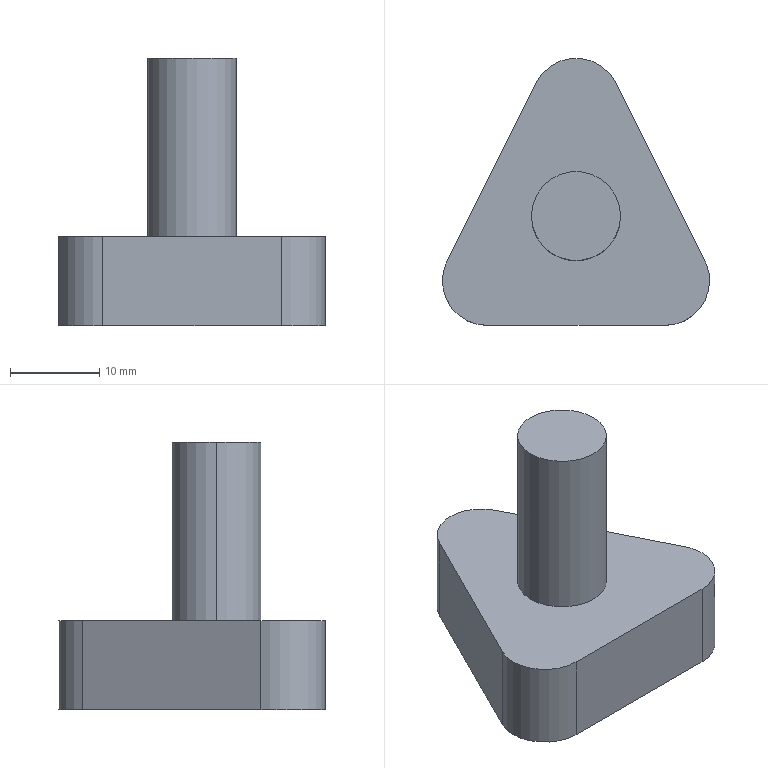Part | STEP file | 1 solid | 12 faces | box 30 x 30 x 30 mm | volume 7592 mm3 | cylinder 6 | plane 6 | commonest cylinder face diameters 10 x6
STEP:
#1=CARTESIAN_POINT('',(0.,0.,0.));
#2=DIRECTION('',(0.,0.,1.));
#3=DIRECTION('',(1.,0.,0.));
#4=AXIS2_PLACEMENT_3D('',#1,#2,#3);
#5=CARTESIAN_POINT('',(5.,-27.762,10.));
#6=VERTEX_POINT('',#5);
#7=CARTESIAN_POINT('',(-5.,-27.762,10.));
#8=VERTEX_POINT('',#7);
#9=CARTESIAN_POINT('',(0.,-27.762,10.));
#10=DIRECTION('',(0.,0.,1.));
#11=DIRECTION('',(1.,0.,0.));
#12=AXIS2_PLACEMENT_3D('',#9,#10,#11);
#13=CIRCLE('',#12,5.);
#14=CARTESIAN_POINT('',(0.,-27.762,10.));
#15=DIRECTION('',(0.,0.,1.));
#16=DIRECTION('',(1.,0.,0.));
#17=AXIS2_PLACEMENT_3D('',#14,#15,#16);
#18=CYLINDRICAL_SURFACE('',#17,5.);
#19=CARTESIAN_POINT('',(0.,0.));
#20=DIRECTION('',(1.,0.));
#21=VECTOR('',#20,1.);
#22=LINE('',#19,#21);
#23=(GEOMETRIC_REPRESENTATION_CONTEXT(2)PARAMETRIC_REPRESENTATION_CONTEXT()REPRESENTATION_CONTEXT('',''));
#24=DEFINITIONAL_REPRESENTATION('',(#22),#23);
#25=PCURVE('',#18,#24);
#26=CARTESIAN_POINT('',(0.,-28.053,10.));
#27=DIRECTION('',(0.,0.,1.));
#28=DIRECTION('',(1.,0.,0.));
#29=AXIS2_PLACEMENT_3D('',#26,#27,#28);
#30=PLANE('',#29);
#31=CARTESIAN_POINT('',(0.,0.2914));
#32=DIRECTION('',(1.,0.));
#33=AXIS2_PLACEMENT_2D('',#31,#32);
#34=CIRCLE('',#33,5.);
#35=(GEOMETRIC_REPRESENTATION_CONTEXT(2)PARAMETRIC_REPRESENTATION_CONTEXT()REPRESENTATION_CONTEXT('',''));
#36=DEFINITIONAL_REPRESENTATION('',(#34),#35);
#37=PCURVE('',#30,#36);
#38=SURFACE_CURVE('',#13,(#25,#37),.PCURVE_S1.);
#39=EDGE_CURVE('',#6,#8,#38,.T.);
#40=ORIENTED_EDGE('',*,*,#39,.T.);
#41=CARTESIAN_POINT('',(-5.,-27.762,30.));
#42=VERTEX_POINT('',#41);
#43=CARTESIAN_POINT('',(-5.,-27.762,10.));
#44=DIRECTION('',(0.,0.,1.));
#45=VECTOR('',#44,1.);
#46=LINE('',#43,#45);
#47=CARTESIAN_POINT('',(3.142,0.));
#48=DIRECTION('',(0.,1.));
#49=VECTOR('',#48,1.);
#50=LINE('',#47,#49);
#51=(GEOMETRIC_REPRESENTATION_CONTEXT(2)PARAMETRIC_REPRESENTATION_CONTEXT()REPRESENTATION_CONTEXT('',''));
#52=DEFINITIONAL_REPRESENTATION('',(#50),#51);
#53=PCURVE('',#18,#52);
#54=CARTESIAN_POINT('',(0.,-27.762,10.));
#55=DIRECTION('',(0.,0.,1.));
#56=DIRECTION('',(1.,0.,0.));
#57=AXIS2_PLACEMENT_3D('',#54,#55,#56);
#58=CYLINDRICAL_SURFACE('',#57,5.);
#59=CARTESIAN_POINT('',(3.142,0.));
#60=DIRECTION('',(0.,1.));
#61=VECTOR('',#60,1.);
#62=LINE('',#59,#61);
#63=(GEOMETRIC_REPRESENTATION_CONTEXT(2)PARAMETRIC_REPRESENTATION_CONTEXT()REPRESENTATION_CONTEXT('',''));
#64=DEFINITIONAL_REPRESENTATION('',(#62),#63);
#65=PCURVE('',#58,#64);
#66=SURFACE_CURVE('',#46,(#53,#65),.PCURVE_S1.);
#67=EDGE_CURVE('',#8,#42,#66,.T.);
#68=ORIENTED_EDGE('',*,*,#67,.T.);
#69=CARTESIAN_POINT('',(5.,-27.762,30.));
#70=VERTEX_POINT('',#69);
#71=CARTESIAN_POINT('',(0.,-27.762,30.));
#72=DIRECTION('',(0.,0.,-1.));
#73=DIRECTION('',(1.,0.,0.));
#74=AXIS2_PLACEMENT_3D('',#71,#72,#73);
#75=CIRCLE('',#74,5.);
#76=CARTESIAN_POINT('',(6.283,20.));
#77=DIRECTION('',(-1.,0.));
#78=VECTOR('',#77,1.);
#79=LINE('',#76,#78);
#80=(GEOMETRIC_REPRESENTATION_CONTEXT(2)PARAMETRIC_REPRESENTATION_CONTEXT()REPRESENTATION_CONTEXT('',''));
#81=DEFINITIONAL_REPRESENTATION('',(#79),#80);
#82=PCURVE('',#18,#81);
#83=CARTESIAN_POINT('',(0.,-27.762,30.));
#84=DIRECTION('',(0.,0.,1.));
#85=DIRECTION('',(1.,0.,0.));
#86=AXIS2_PLACEMENT_3D('',#83,#84,#85);
#87=PLANE('',#86);
#88=CARTESIAN_POINT('',(5.,0.));
#89=CARTESIAN_POINT('',(5.,-8.66));
#90=CARTESIAN_POINT('',(-2.5,-4.33));
#91=CARTESIAN_POINT('',(-10.,0.));
#92=CARTESIAN_POINT('',(-2.5,4.33));
#93=CARTESIAN_POINT('',(5.,8.66));
#94=CARTESIAN_POINT('',(5.,0.));
#95=(BOUNDED_CURVE()B_SPLINE_CURVE(2,(#88,#89,#90,#91,#92,#93,#94),.UNSPECIFIED.,.T.,.F.)B_SPLINE_CURVE_WITH_KNOTS((1,2,2,2,2,1),(-2.094,0.,2.094,4.189,6.283,8.378),.UNSPECIFIED.)CURVE()GEOMETRIC_REPRESENTATION_ITEM()RATIONAL_B_SPLINE_CURVE((1.,0.5,1.,0.5,1.,0.5,1.))REPRESENTATION_ITEM(''));
#96=(GEOMETRIC_REPRESENTATION_CONTEXT(2)PARAMETRIC_REPRESENTATION_CONTEXT()REPRESENTATION_CONTEXT('',''));
#97=DEFINITIONAL_REPRESENTATION('',(#95),#96);
#98=PCURVE('',#87,#97);
#99=SURFACE_CURVE('',#75,(#82,#98),.PCURVE_S1.);
#100=EDGE_CURVE('',#42,#70,#99,.T.);
#101=ORIENTED_EDGE('',*,*,#100,.T.);
#102=CARTESIAN_POINT('',(5.,-27.762,10.));
#103=DIRECTION('',(0.,0.,1.));
#104=VECTOR('',#103,1.);
#105=LINE('',#102,#104);
#106=CARTESIAN_POINT('',(0.,0.));
#107=DIRECTION('',(0.,1.));
#108=VECTOR('',#107,1.);
#109=LINE('',#106,#108);
#110=(GEOMETRIC_REPRESENTATION_CONTEXT(2)PARAMETRIC_REPRESENTATION_CONTEXT()REPRESENTATION_CONTEXT('',''));
#111=DEFINITIONAL_REPRESENTATION('',(#109),#110);
#112=PCURVE('',#18,#111);
#113=CARTESIAN_POINT('',(6.283,0.));
#114=DIRECTION('',(0.,1.));
#115=VECTOR('',#114,1.);
#116=LINE('',#113,#115);
#117=(GEOMETRIC_REPRESENTATION_CONTEXT(2)PARAMETRIC_REPRESENTATION_CONTEXT()REPRESENTATION_CONTEXT('',''));
#118=DEFINITIONAL_REPRESENTATION('',(#116),#117);
#119=PCURVE('',#58,#118);
#120=SURFACE_CURVE('',#105,(#112,#119),.PCURVE_S1.);
#121=EDGE_CURVE('',#6,#70,#120,.T.);
#122=ORIENTED_EDGE('',*,*,#121,.F.);
#123=EDGE_LOOP('',(#40,#68,#101,#122));
#124=FACE_BOUND('',#123,.T.);
#125=ADVANCED_FACE('',(#124),#18,.T.);
#126=CARTESIAN_POINT('',(10.,-40.,0.));
#127=VERTEX_POINT('',#126);
#128=CARTESIAN_POINT('',(15.,-35.,0.));
#129=VERTEX_POINT('',#128);
#130=CARTESIAN_POINT('',(10.,-35.,0.));
#131=DIRECTION('',(0.,0.,1.));
#132=DIRECTION('',(1.,0.,0.));
#133=AXIS2_PLACEMENT_3D('',#130,#131,#132);
#134=CIRCLE('',#133,5.);
#135=CARTESIAN_POINT('',(10.,-35.,0.));
#136=DIRECTION('',(0.,0.,1.));
#137=DIRECTION('',(1.,0.,0.));
#138=AXIS2_PLACEMENT_3D('',#135,#136,#137);
#139=CYLINDRICAL_SURFACE('',#138,5.);
#140=CARTESIAN_POINT('',(0.,0.));
#141=DIRECTION('',(1.,0.));
#142=VECTOR('',#141,1.);
#143=LINE('',#140,#142);
#144=(GEOMETRIC_REPRESENTATION_CONTEXT(2)PARAMETRIC_REPRESENTATION_CONTEXT()REPRESENTATION_CONTEXT('',''));
#145=DEFINITIONAL_REPRESENTATION('',(#143),#144);
#146=PCURVE('',#139,#145);
#147=CARTESIAN_POINT('',(0.,-28.053,0.));
#148=DIRECTION('',(0.,0.,1.));
#149=DIRECTION('',(1.,0.,0.));
#150=AXIS2_PLACEMENT_3D('',#147,#148,#149);
#151=PLANE('',#150);
#152=CARTESIAN_POINT('',(10.,-6.947));
#153=DIRECTION('',(1.,0.));
#154=AXIS2_PLACEMENT_2D('',#152,#153);
#155=CIRCLE('',#154,5.);
#156=(GEOMETRIC_REPRESENTATION_CONTEXT(2)PARAMETRIC_REPRESENTATION_CONTEXT()REPRESENTATION_CONTEXT('',''));
#157=DEFINITIONAL_REPRESENTATION('',(#155),#156);
#158=PCURVE('',#151,#157);
#159=SURFACE_CURVE('',#134,(#146,#158),.PCURVE_S1.);
#160=EDGE_CURVE('',#127,#129,#159,.T.);
#161=ORIENTED_EDGE('',*,*,#160,.T.);
#162=CARTESIAN_POINT('',(15.,-35.,10.));
#163=VERTEX_POINT('',#162);
#164=CARTESIAN_POINT('',(15.,-35.,0.));
#165=DIRECTION('',(0.,0.,1.));
#166=VECTOR('',#165,1.);
#167=LINE('',#164,#166);
#168=CARTESIAN_POINT('',(6.283,0.));
#169=DIRECTION('',(0.,1.));
#170=VECTOR('',#169,1.);
#171=LINE('',#168,#170);
#172=(GEOMETRIC_REPRESENTATION_CONTEXT(2)PARAMETRIC_REPRESENTATION_CONTEXT()REPRESENTATION_CONTEXT('',''));
#173=DEFINITIONAL_REPRESENTATION('',(#171),#172);
#174=PCURVE('',#139,#173);
#175=CARTESIAN_POINT('',(10.,-35.,0.));
#176=DIRECTION('',(0.,0.,1.));
#177=DIRECTION('',(1.,0.,0.));
#178=AXIS2_PLACEMENT_3D('',#175,#176,#177);
#179=CYLINDRICAL_SURFACE('',#178,5.);
#180=CARTESIAN_POINT('',(0.,0.));
#181=DIRECTION('',(0.,1.));
#182=VECTOR('',#181,1.);
#183=LINE('',#180,#182);
#184=(GEOMETRIC_REPRESENTATION_CONTEXT(2)PARAMETRIC_REPRESENTATION_CONTEXT()REPRESENTATION_CONTEXT('',''));
#185=DEFINITIONAL_REPRESENTATION('',(#183),#184);
#186=PCURVE('',#179,#185);
#187=SURFACE_CURVE('',#167,(#174,#186),.PCURVE_S1.);
#188=EDGE_CURVE('',#129,#163,#187,.T.);
#189=ORIENTED_EDGE('',*,*,#188,.T.);
#190=CARTESIAN_POINT('',(10.,-40.,10.));
#191=VERTEX_POINT('',#190);
#192=CARTESIAN_POINT('',(10.,-35.,10.));
#193=DIRECTION('',(0.,0.,1.));
#194=DIRECTION('',(1.,0.,0.));
#195=AXIS2_PLACEMENT_3D('',#192,#193,#194);
#196=CIRCLE('',#195,5.);
#197=CARTESIAN_POINT('',(0.,10.));
#198=DIRECTION('',(1.,0.));
#199=VECTOR('',#198,1.);
#200=LINE('',#197,#199);
#201=(GEOMETRIC_REPRESENTATION_CONTEXT(2)PARAMETRIC_REPRESENTATION_CONTEXT()REPRESENTATION_CONTEXT('',''));
#202=DEFINITIONAL_REPRESENTATION('',(#200),#201);
#203=PCURVE('',#139,#202);
#204=CARTESIAN_POINT('',(10.,-6.947));
#205=DIRECTION('',(1.,0.));
#206=AXIS2_PLACEMENT_2D('',#204,#205);
#207=CIRCLE('',#206,5.);
#208=(GEOMETRIC_REPRESENTATION_CONTEXT(2)PARAMETRIC_REPRESENTATION_CONTEXT()REPRESENTATION_CONTEXT('',''));
#209=DEFINITIONAL_REPRESENTATION('',(#207),#208);
#210=PCURVE('',#30,#209);
#211=SURFACE_CURVE('',#196,(#203,#210),.PCURVE_S1.);
#212=EDGE_CURVE('',#191,#163,#211,.T.);
#213=ORIENTED_EDGE('',*,*,#212,.F.);
#214=CARTESIAN_POINT('',(10.,-40.,0.));
#215=DIRECTION('',(0.,0.,-1.));
#216=VECTOR('',#215,1.);
#217=LINE('',#214,#216);
#218=CARTESIAN_POINT('',(4.712,0.));
#219=DIRECTION('',(0.,-1.));
#220=VECTOR('',#219,1.);
#221=LINE('',#218,#220);
#222=(GEOMETRIC_REPRESENTATION_CONTEXT(2)PARAMETRIC_REPRESENTATION_CONTEXT()REPRESENTATION_CONTEXT('',''));
#223=DEFINITIONAL_REPRESENTATION('',(#221),#222);
#224=PCURVE('',#139,#223);
#225=CARTESIAN_POINT('',(-10.,-40.,0.));
#226=DIRECTION('',(0.,-1.,0.));
#227=DIRECTION('',(0.,0.,-1.));
#228=AXIS2_PLACEMENT_3D('',#225,#226,#227);
#229=PLANE('',#228);
#230=CARTESIAN_POINT('',(0.,20.));
#231=DIRECTION('',(1.,0.));
#232=VECTOR('',#231,1.);
#233=LINE('',#230,#232);
#234=(GEOMETRIC_REPRESENTATION_CONTEXT(2)PARAMETRIC_REPRESENTATION_CONTEXT()REPRESENTATION_CONTEXT('',''));
#235=DEFINITIONAL_REPRESENTATION('',(#233),#234);
#236=PCURVE('',#229,#235);
#237=SURFACE_CURVE('',#217,(#224,#236),.PCURVE_S1.);
#238=EDGE_CURVE('',#191,#127,#237,.T.);
#239=ORIENTED_EDGE('',*,*,#238,.T.);
#240=EDGE_LOOP('',(#161,#189,#213,#239));
#241=FACE_BOUND('',#240,.T.);
#242=ADVANCED_FACE('',(#241),#139,.T.);
#243=ORIENTED_EDGE('',*,*,#67,.F.);
#244=CARTESIAN_POINT('',(0.,-27.762,10.));
#245=DIRECTION('',(0.,0.,1.));
#246=DIRECTION('',(1.,0.,0.));
#247=AXIS2_PLACEMENT_3D('',#244,#245,#246);
#248=CIRCLE('',#247,5.);
#249=CARTESIAN_POINT('',(0.,0.));
#250=DIRECTION('',(1.,0.));
#251=VECTOR('',#250,1.);
#252=LINE('',#249,#251);
#253=(GEOMETRIC_REPRESENTATION_CONTEXT(2)PARAMETRIC_REPRESENTATION_CONTEXT()REPRESENTATION_CONTEXT('',''));
#254=DEFINITIONAL_REPRESENTATION('',(#252),#253);
#255=PCURVE('',#58,#254);
#256=CARTESIAN_POINT('',(0.,0.2914));
#257=DIRECTION('',(1.,0.));
#258=AXIS2_PLACEMENT_2D('',#256,#257);
#259=CIRCLE('',#258,5.);
#260=(GEOMETRIC_REPRESENTATION_CONTEXT(2)PARAMETRIC_REPRESENTATION_CONTEXT()REPRESENTATION_CONTEXT('',''));
#261=DEFINITIONAL_REPRESENTATION('',(#259),#260);
#262=PCURVE('',#30,#261);
#263=SURFACE_CURVE('',#248,(#255,#262),.PCURVE_S1.);
#264=EDGE_CURVE('',#8,#6,#263,.T.);
#265=ORIENTED_EDGE('',*,*,#264,.T.);
#266=ORIENTED_EDGE('',*,*,#121,.T.);
#267=CARTESIAN_POINT('',(0.,-27.762,30.));
#268=DIRECTION('',(0.,0.,-1.));
#269=DIRECTION('',(1.,0.,0.));
#270=AXIS2_PLACEMENT_3D('',#267,#268,#269);
#271=CIRCLE('',#270,5.);
#272=CARTESIAN_POINT('',(6.283,20.));
#273=DIRECTION('',(-1.,0.));
#274=VECTOR('',#273,1.);
#275=LINE('',#272,#274);
#276=(GEOMETRIC_REPRESENTATION_CONTEXT(2)PARAMETRIC_REPRESENTATION_CONTEXT()REPRESENTATION_CONTEXT('',''));
#277=DEFINITIONAL_REPRESENTATION('',(#275),#276);
#278=PCURVE('',#58,#277);
#279=CARTESIAN_POINT('',(5.,0.));
#280=CARTESIAN_POINT('',(5.,-8.66));
#281=CARTESIAN_POINT('',(-2.5,-4.33));
#282=CARTESIAN_POINT('',(-10.,0.));
#283=CARTESIAN_POINT('',(-2.5,4.33));
#284=CARTESIAN_POINT('',(5.,8.66));
#285=CARTESIAN_POINT('',(5.,0.));
#286=(BOUNDED_CURVE()B_SPLINE_CURVE(2,(#279,#280,#281,#282,#283,#284,#285),.UNSPECIFIED.,.T.,.F.)B_SPLINE_CURVE_WITH_KNOTS((1,2,2,2,2,1),(-2.094,0.,2.094,4.189,6.283,8.378),.UNSPECIFIED.)CURVE()GEOMETRIC_REPRESENTATION_ITEM()RATIONAL_B_SPLINE_CURVE((1.,0.5,1.,0.5,1.,0.5,1.))REPRESENTATION_ITEM(''));
#287=(GEOMETRIC_REPRESENTATION_CONTEXT(2)PARAMETRIC_REPRESENTATION_CONTEXT()REPRESENTATION_CONTEXT('',''));
#288=DEFINITIONAL_REPRESENTATION('',(#286),#287);
#289=PCURVE('',#87,#288);
#290=SURFACE_CURVE('',#271,(#278,#289),.PCURVE_S1.);
#291=EDGE_CURVE('',#70,#42,#290,.T.);
#292=ORIENTED_EDGE('',*,*,#291,.T.);
#293=EDGE_LOOP('',(#243,#265,#266,#292));
#294=FACE_BOUND('',#293,.T.);
#295=ADVANCED_FACE('',(#294),#58,.T.);
#296=CARTESIAN_POINT('',(-10.,-40.,10.));
#297=VERTEX_POINT('',#296);
#298=CARTESIAN_POINT('',(0.,-40.,10.));
#299=DIRECTION('',(1.,0.,0.));
#300=VECTOR('',#299,1.);
#301=LINE('',#298,#300);
#302=CARTESIAN_POINT('',(0.,-11.947));
#303=DIRECTION('',(1.,0.));
#304=VECTOR('',#303,1.);
#305=LINE('',#302,#304);
#306=(GEOMETRIC_REPRESENTATION_CONTEXT(2)PARAMETRIC_REPRESENTATION_CONTEXT()REPRESENTATION_CONTEXT('',''));
#307=DEFINITIONAL_REPRESENTATION('',(#305),#306);
#308=PCURVE('',#30,#307);
#309=CARTESIAN_POINT('',(-10.,10.));
#310=DIRECTION('',(0.,1.));
#311=VECTOR('',#310,1.);
#312=LINE('',#309,#311);
#313=(GEOMETRIC_REPRESENTATION_CONTEXT(2)PARAMETRIC_REPRESENTATION_CONTEXT()REPRESENTATION_CONTEXT('',''));
#314=DEFINITIONAL_REPRESENTATION('',(#312),#313);
#315=PCURVE('',#229,#314);
#316=SURFACE_CURVE('',#301,(#308,#315),.PCURVE_S1.);
#317=EDGE_CURVE('',#297,#191,#316,.T.);
#318=ORIENTED_EDGE('',*,*,#317,.T.);
#319=ORIENTED_EDGE('',*,*,#212,.T.);
#320=CARTESIAN_POINT('',(14.472,-32.764,10.));
#321=VERTEX_POINT('',#320);
#322=CARTESIAN_POINT('',(10.,-35.,10.));
#323=DIRECTION('',(0.,0.,1.));
#324=DIRECTION('',(1.,0.,0.));
#325=AXIS2_PLACEMENT_3D('',#322,#323,#324);
#326=CIRCLE('',#325,5.);
#327=CARTESIAN_POINT('',(10.,-6.947));
#328=DIRECTION('',(1.,0.));
#329=AXIS2_PLACEMENT_2D('',#327,#328);
#330=CIRCLE('',#329,5.);
#331=(GEOMETRIC_REPRESENTATION_CONTEXT(2)PARAMETRIC_REPRESENTATION_CONTEXT()REPRESENTATION_CONTEXT('',''));
#332=DEFINITIONAL_REPRESENTATION('',(#330),#331);
#333=PCURVE('',#30,#332);
#334=CARTESIAN_POINT('',(0.,10.));
#335=DIRECTION('',(1.,0.));
#336=VECTOR('',#335,1.);
#337=LINE('',#334,#336);
#338=(GEOMETRIC_REPRESENTATION_CONTEXT(2)PARAMETRIC_REPRESENTATION_CONTEXT()REPRESENTATION_CONTEXT('',''));
#339=DEFINITIONAL_REPRESENTATION('',(#337),#338);
#340=PCURVE('',#179,#339);
#341=SURFACE_CURVE('',#326,(#333,#340),.PCURVE_S1.);
#342=EDGE_CURVE('',#163,#321,#341,.T.);
#343=ORIENTED_EDGE('',*,*,#342,.T.);
#344=CARTESIAN_POINT('',(4.472,-12.764,10.));
#345=VERTEX_POINT('',#344);
#346=CARTESIAN_POINT('',(14.472,-32.764,10.));
#347=DIRECTION('',(-0.4472,0.8944,0.));
#348=VECTOR('',#347,1.);
#349=LINE('',#346,#348);
#350=CARTESIAN_POINT('',(14.472,-4.711));
#351=DIRECTION('',(-0.4472,0.8944));
#352=VECTOR('',#351,1.);
#353=LINE('',#350,#352);
#354=(GEOMETRIC_REPRESENTATION_CONTEXT(2)PARAMETRIC_REPRESENTATION_CONTEXT()REPRESENTATION_CONTEXT('',''));
#355=DEFINITIONAL_REPRESENTATION('',(#353),#354);
#356=PCURVE('',#30,#355);
#357=CARTESIAN_POINT('',(14.472,-32.764,0.));
#358=DIRECTION('',(0.8944,0.4472,0.));
#359=DIRECTION('',(-0.4472,0.8944,0.));
#360=AXIS2_PLACEMENT_3D('',#357,#358,#359);
#361=PLANE('',#360);
#362=CARTESIAN_POINT('',(0.,10.));
#363=DIRECTION('',(1.,0.));
#364=VECTOR('',#363,1.);
#365=LINE('',#362,#364);
#366=(GEOMETRIC_REPRESENTATION_CONTEXT(2)PARAMETRIC_REPRESENTATION_CONTEXT()REPRESENTATION_CONTEXT('',''));
#367=DEFINITIONAL_REPRESENTATION('',(#365),#366);
#368=PCURVE('',#361,#367);
#369=SURFACE_CURVE('',#349,(#356,#368),.PCURVE_S1.);
#370=EDGE_CURVE('',#321,#345,#369,.T.);
#371=ORIENTED_EDGE('',*,*,#370,.T.);
#372=CARTESIAN_POINT('',(-4.472,-12.764,10.));
#373=VERTEX_POINT('',#372);
#374=CARTESIAN_POINT('',(0.,-15.,10.));
#375=DIRECTION('',(0.,0.,1.));
#376=DIRECTION('',(1.,0.,0.));
#377=AXIS2_PLACEMENT_3D('',#374,#375,#376);
#378=CIRCLE('',#377,5.);
#379=CARTESIAN_POINT('',(0.,13.053));
#380=DIRECTION('',(1.,0.));
#381=AXIS2_PLACEMENT_2D('',#379,#380);
#382=CIRCLE('',#381,5.);
#383=(GEOMETRIC_REPRESENTATION_CONTEXT(2)PARAMETRIC_REPRESENTATION_CONTEXT()REPRESENTATION_CONTEXT('',''));
#384=DEFINITIONAL_REPRESENTATION('',(#382),#383);
#385=PCURVE('',#30,#384);
#386=CARTESIAN_POINT('',(0.,-15.,0.));
#387=DIRECTION('',(0.,0.,1.));
#388=DIRECTION('',(1.,0.,0.));
#389=AXIS2_PLACEMENT_3D('',#386,#387,#388);
#390=CYLINDRICAL_SURFACE('',#389,5.);
#391=CARTESIAN_POINT('',(0.,10.));
#392=DIRECTION('',(1.,0.));
#393=VECTOR('',#392,1.);
#394=LINE('',#391,#393);
#395=(GEOMETRIC_REPRESENTATION_CONTEXT(2)PARAMETRIC_REPRESENTATION_CONTEXT()REPRESENTATION_CONTEXT('',''));
#396=DEFINITIONAL_REPRESENTATION('',(#394),#395);
#397=PCURVE('',#390,#396);
#398=SURFACE_CURVE('',#378,(#385,#397),.PCURVE_S1.);
#399=EDGE_CURVE('',#345,#373,#398,.T.);
#400=ORIENTED_EDGE('',*,*,#399,.T.);
#401=CARTESIAN_POINT('',(-14.472,-32.764,10.));
#402=VERTEX_POINT('',#401);
#403=CARTESIAN_POINT('',(-4.472,-12.764,10.));
#404=DIRECTION('',(-0.4472,-0.8944,0.));
#405=VECTOR('',#404,1.);
#406=LINE('',#403,#405);
#407=CARTESIAN_POINT('',(-4.472,15.289));
#408=DIRECTION('',(-0.4472,-0.8944));
#409=VECTOR('',#408,1.);
#410=LINE('',#407,#409);
#411=(GEOMETRIC_REPRESENTATION_CONTEXT(2)PARAMETRIC_REPRESENTATION_CONTEXT()REPRESENTATION_CONTEXT('',''));
#412=DEFINITIONAL_REPRESENTATION('',(#410),#411);
#413=PCURVE('',#30,#412);
#414=CARTESIAN_POINT('',(-4.472,-12.764,0.));
#415=DIRECTION('',(-0.8944,0.4472,0.));
#416=DIRECTION('',(-0.4472,-0.8944,0.));
#417=AXIS2_PLACEMENT_3D('',#414,#415,#416);
#418=PLANE('',#417);
#419=CARTESIAN_POINT('',(0.,10.));
#420=DIRECTION('',(1.,0.));
#421=VECTOR('',#420,1.);
#422=LINE('',#419,#421);
#423=(GEOMETRIC_REPRESENTATION_CONTEXT(2)PARAMETRIC_REPRESENTATION_CONTEXT()REPRESENTATION_CONTEXT('',''));
#424=DEFINITIONAL_REPRESENTATION('',(#422),#423);
#425=PCURVE('',#418,#424);
#426=SURFACE_CURVE('',#406,(#413,#425),.PCURVE_S1.);
#427=EDGE_CURVE('',#373,#402,#426,.T.);
#428=ORIENTED_EDGE('',*,*,#427,.T.);
#429=CARTESIAN_POINT('',(-10.,-35.,10.));
#430=DIRECTION('',(0.,0.,1.));
#431=DIRECTION('',(1.,0.,0.));
#432=AXIS2_PLACEMENT_3D('',#429,#430,#431);
#433=CIRCLE('',#432,5.);
#434=CARTESIAN_POINT('',(-10.,-6.947));
#435=DIRECTION('',(1.,0.));
#436=AXIS2_PLACEMENT_2D('',#434,#435);
#437=CIRCLE('',#436,5.);
#438=(GEOMETRIC_REPRESENTATION_CONTEXT(2)PARAMETRIC_REPRESENTATION_CONTEXT()REPRESENTATION_CONTEXT('',''));
#439=DEFINITIONAL_REPRESENTATION('',(#437),#438);
#440=PCURVE('',#30,#439);
#441=CARTESIAN_POINT('',(-10.,-35.,0.));
#442=DIRECTION('',(0.,0.,1.));
#443=DIRECTION('',(1.,0.,0.));
#444=AXIS2_PLACEMENT_3D('',#441,#442,#443);
#445=CYLINDRICAL_SURFACE('',#444,5.);
#446=CARTESIAN_POINT('',(0.,10.));
#447=DIRECTION('',(1.,0.));
#448=VECTOR('',#447,1.);
#449=LINE('',#446,#448);
#450=(GEOMETRIC_REPRESENTATION_CONTEXT(2)PARAMETRIC_REPRESENTATION_CONTEXT()REPRESENTATION_CONTEXT('',''));
#451=DEFINITIONAL_REPRESENTATION('',(#449),#450);
#452=PCURVE('',#445,#451);
#453=SURFACE_CURVE('',#433,(#440,#452),.PCURVE_S1.);
#454=EDGE_CURVE('',#402,#297,#453,.T.);
#455=ORIENTED_EDGE('',*,*,#454,.T.);
#456=EDGE_LOOP('',(#318,#319,#343,#371,#400,#428,#455));
#457=FACE_BOUND('',#456,.T.);
#458=ORIENTED_EDGE('',*,*,#39,.F.);
#459=ORIENTED_EDGE('',*,*,#264,.F.);
#460=EDGE_LOOP('',(#458,#459));
#461=FACE_BOUND('',#460,.T.);
#462=ADVANCED_FACE('',(#457,#461),#30,.T.);
#463=ORIENTED_EDGE('',*,*,#291,.F.);
#464=ORIENTED_EDGE('',*,*,#100,.F.);
#465=EDGE_LOOP('',(#463,#464));
#466=FACE_BOUND('',#465,.T.);
#467=ADVANCED_FACE('',(#466),#87,.T.);
#468=ORIENTED_EDGE('',*,*,#188,.F.);
#469=CARTESIAN_POINT('',(14.472,-32.764,0.));
#470=VERTEX_POINT('',#469);
#471=CARTESIAN_POINT('',(10.,-35.,0.));
#472=DIRECTION('',(0.,0.,1.));
#473=DIRECTION('',(1.,0.,0.));
#474=AXIS2_PLACEMENT_3D('',#471,#472,#473);
#475=CIRCLE('',#474,5.);
#476=CARTESIAN_POINT('',(0.,0.));
#477=DIRECTION('',(1.,0.));
#478=VECTOR('',#477,1.);
#479=LINE('',#476,#478);
#480=(GEOMETRIC_REPRESENTATION_CONTEXT(2)PARAMETRIC_REPRESENTATION_CONTEXT()REPRESENTATION_CONTEXT('',''));
#481=DEFINITIONAL_REPRESENTATION('',(#479),#480);
#482=PCURVE('',#179,#481);
#483=CARTESIAN_POINT('',(10.,-6.947));
#484=DIRECTION('',(1.,0.));
#485=AXIS2_PLACEMENT_2D('',#483,#484);
#486=CIRCLE('',#485,5.);
#487=(GEOMETRIC_REPRESENTATION_CONTEXT(2)PARAMETRIC_REPRESENTATION_CONTEXT()REPRESENTATION_CONTEXT('',''));
#488=DEFINITIONAL_REPRESENTATION('',(#486),#487);
#489=PCURVE('',#151,#488);
#490=SURFACE_CURVE('',#475,(#482,#489),.PCURVE_S1.);
#491=EDGE_CURVE('',#129,#470,#490,.T.);
#492=ORIENTED_EDGE('',*,*,#491,.T.);
#493=CARTESIAN_POINT('',(14.472,-32.764,0.));
#494=DIRECTION('',(0.,0.,1.));
#495=VECTOR('',#494,1.);
#496=LINE('',#493,#495);
#497=CARTESIAN_POINT('',(0.4636,0.));
#498=DIRECTION('',(0.,1.));
#499=VECTOR('',#498,1.);
#500=LINE('',#497,#499);
#501=(GEOMETRIC_REPRESENTATION_CONTEXT(2)PARAMETRIC_REPRESENTATION_CONTEXT()REPRESENTATION_CONTEXT('',''));
#502=DEFINITIONAL_REPRESENTATION('',(#500),#501);
#503=PCURVE('',#179,#502);
#504=CARTESIAN_POINT('',(0.,0.));
#505=DIRECTION('',(0.,1.));
#506=VECTOR('',#505,1.);
#507=LINE('',#504,#506);
#508=(GEOMETRIC_REPRESENTATION_CONTEXT(2)PARAMETRIC_REPRESENTATION_CONTEXT()REPRESENTATION_CONTEXT('',''));
#509=DEFINITIONAL_REPRESENTATION('',(#507),#508);
#510=PCURVE('',#361,#509);
#511=SURFACE_CURVE('',#496,(#503,#510),.PCURVE_S1.);
#512=EDGE_CURVE('',#470,#321,#511,.T.);
#513=ORIENTED_EDGE('',*,*,#512,.T.);
#514=ORIENTED_EDGE('',*,*,#342,.F.);
#515=EDGE_LOOP('',(#468,#492,#513,#514));
#516=FACE_BOUND('',#515,.T.);
#517=ADVANCED_FACE('',(#516),#179,.T.);
#518=ORIENTED_EDGE('',*,*,#317,.F.);
#519=CARTESIAN_POINT('',(-10.,-40.,0.));
#520=VERTEX_POINT('',#519);
#521=CARTESIAN_POINT('',(-10.,-40.,0.));
#522=DIRECTION('',(0.,0.,-1.));
#523=VECTOR('',#522,1.);
#524=LINE('',#521,#523);
#525=CARTESIAN_POINT('',(0.,0.));
#526=DIRECTION('',(1.,0.));
#527=VECTOR('',#526,1.);
#528=LINE('',#525,#527);
#529=(GEOMETRIC_REPRESENTATION_CONTEXT(2)PARAMETRIC_REPRESENTATION_CONTEXT()REPRESENTATION_CONTEXT('',''));
#530=DEFINITIONAL_REPRESENTATION('',(#528),#529);
#531=PCURVE('',#229,#530);
#532=CARTESIAN_POINT('',(4.712,0.));
#533=DIRECTION('',(0.,-1.));
#534=VECTOR('',#533,1.);
#535=LINE('',#532,#534);
#536=(GEOMETRIC_REPRESENTATION_CONTEXT(2)PARAMETRIC_REPRESENTATION_CONTEXT()REPRESENTATION_CONTEXT('',''));
#537=DEFINITIONAL_REPRESENTATION('',(#535),#536);
#538=PCURVE('',#445,#537);
#539=SURFACE_CURVE('',#524,(#531,#538),.PCURVE_S1.);
#540=EDGE_CURVE('',#297,#520,#539,.T.);
#541=ORIENTED_EDGE('',*,*,#540,.T.);
#542=CARTESIAN_POINT('',(-10.,-40.,0.));
#543=DIRECTION('',(1.,0.,0.));
#544=VECTOR('',#543,1.);
#545=LINE('',#542,#544);
#546=CARTESIAN_POINT('',(0.,0.));
#547=DIRECTION('',(0.,1.));
#548=VECTOR('',#547,1.);
#549=LINE('',#546,#548);
#550=(GEOMETRIC_REPRESENTATION_CONTEXT(2)PARAMETRIC_REPRESENTATION_CONTEXT()REPRESENTATION_CONTEXT('',''));
#551=DEFINITIONAL_REPRESENTATION('',(#549),#550);
#552=PCURVE('',#229,#551);
#553=CARTESIAN_POINT('',(-10.,-11.947));
#554=DIRECTION('',(1.,0.));
#555=VECTOR('',#554,1.);
#556=LINE('',#553,#555);
#557=(GEOMETRIC_REPRESENTATION_CONTEXT(2)PARAMETRIC_REPRESENTATION_CONTEXT()REPRESENTATION_CONTEXT('',''));
#558=DEFINITIONAL_REPRESENTATION('',(#556),#557);
#559=PCURVE('',#151,#558);
#560=SURFACE_CURVE('',#545,(#552,#559),.PCURVE_S1.);
#561=EDGE_CURVE('',#520,#127,#560,.T.);
#562=ORIENTED_EDGE('',*,*,#561,.T.);
#563=ORIENTED_EDGE('',*,*,#238,.F.);
#564=EDGE_LOOP('',(#518,#541,#562,#563));
#565=FACE_BOUND('',#564,.T.);
#566=ADVANCED_FACE('',(#565),#229,.T.);
#567=ORIENTED_EDGE('',*,*,#454,.F.);
#568=CARTESIAN_POINT('',(-14.472,-32.764,0.));
#569=VERTEX_POINT('',#568);
#570=CARTESIAN_POINT('',(-14.472,-32.764,0.));
#571=DIRECTION('',(0.,0.,-1.));
#572=VECTOR('',#571,1.);
#573=LINE('',#570,#572);
#574=CARTESIAN_POINT('',(2.678,0.));
#575=DIRECTION('',(0.,-1.));
#576=VECTOR('',#575,1.);
#577=LINE('',#574,#576);
#578=(GEOMETRIC_REPRESENTATION_CONTEXT(2)PARAMETRIC_REPRESENTATION_CONTEXT()REPRESENTATION_CONTEXT('',''));
#579=DEFINITIONAL_REPRESENTATION('',(#577),#578);
#580=PCURVE('',#445,#579);
#581=CARTESIAN_POINT('',(22.361,0.));
#582=DIRECTION('',(0.,-1.));
#583=VECTOR('',#582,1.);
#584=LINE('',#581,#583);
#585=(GEOMETRIC_REPRESENTATION_CONTEXT(2)PARAMETRIC_REPRESENTATION_CONTEXT()REPRESENTATION_CONTEXT('',''));
#586=DEFINITIONAL_REPRESENTATION('',(#584),#585);
#587=PCURVE('',#418,#586);
#588=SURFACE_CURVE('',#573,(#580,#587),.PCURVE_S1.);
#589=EDGE_CURVE('',#402,#569,#588,.T.);
#590=ORIENTED_EDGE('',*,*,#589,.T.);
#591=CARTESIAN_POINT('',(-10.,-35.,0.));
#592=DIRECTION('',(0.,0.,1.));
#593=DIRECTION('',(1.,0.,0.));
#594=AXIS2_PLACEMENT_3D('',#591,#592,#593);
#595=CIRCLE('',#594,5.);
#596=CARTESIAN_POINT('',(0.,0.));
#597=DIRECTION('',(1.,0.));
#598=VECTOR('',#597,1.);
#599=LINE('',#596,#598);
#600=(GEOMETRIC_REPRESENTATION_CONTEXT(2)PARAMETRIC_REPRESENTATION_CONTEXT()REPRESENTATION_CONTEXT('',''));
#601=DEFINITIONAL_REPRESENTATION('',(#599),#600);
#602=PCURVE('',#445,#601);
#603=CARTESIAN_POINT('',(-10.,-6.947));
#604=DIRECTION('',(1.,0.));
#605=AXIS2_PLACEMENT_2D('',#603,#604);
#606=CIRCLE('',#605,5.);
#607=(GEOMETRIC_REPRESENTATION_CONTEXT(2)PARAMETRIC_REPRESENTATION_CONTEXT()REPRESENTATION_CONTEXT('',''));
#608=DEFINITIONAL_REPRESENTATION('',(#606),#607);
#609=PCURVE('',#151,#608);
#610=SURFACE_CURVE('',#595,(#602,#609),.PCURVE_S1.);
#611=EDGE_CURVE('',#569,#520,#610,.T.);
#612=ORIENTED_EDGE('',*,*,#611,.T.);
#613=ORIENTED_EDGE('',*,*,#540,.F.);
#614=EDGE_LOOP('',(#567,#590,#612,#613));
#615=FACE_BOUND('',#614,.T.);
#616=ADVANCED_FACE('',(#615),#445,.T.);
#617=ORIENTED_EDGE('',*,*,#427,.F.);
#618=CARTESIAN_POINT('',(-4.472,-12.764,0.));
#619=VERTEX_POINT('',#618);
#620=CARTESIAN_POINT('',(-4.472,-12.764,0.));
#621=DIRECTION('',(0.,0.,-1.));
#622=VECTOR('',#621,1.);
#623=LINE('',#620,#622);
#624=CARTESIAN_POINT('',(0.,0.));
#625=DIRECTION('',(0.,-1.));
#626=VECTOR('',#625,1.);
#627=LINE('',#624,#626);
#628=(GEOMETRIC_REPRESENTATION_CONTEXT(2)PARAMETRIC_REPRESENTATION_CONTEXT()REPRESENTATION_CONTEXT('',''));
#629=DEFINITIONAL_REPRESENTATION('',(#627),#628);
#630=PCURVE('',#418,#629);
#631=CARTESIAN_POINT('',(2.678,0.));
#632=DIRECTION('',(0.,-1.));
#633=VECTOR('',#632,1.);
#634=LINE('',#631,#633);
#635=(GEOMETRIC_REPRESENTATION_CONTEXT(2)PARAMETRIC_REPRESENTATION_CONTEXT()REPRESENTATION_CONTEXT('',''));
#636=DEFINITIONAL_REPRESENTATION('',(#634),#635);
#637=PCURVE('',#390,#636);
#638=SURFACE_CURVE('',#623,(#630,#637),.PCURVE_S1.);
#639=EDGE_CURVE('',#373,#619,#638,.T.);
#640=ORIENTED_EDGE('',*,*,#639,.T.);
#641=CARTESIAN_POINT('',(-4.472,-12.764,0.));
#642=DIRECTION('',(-0.4472,-0.8944,0.));
#643=VECTOR('',#642,1.);
#644=LINE('',#641,#643);
#645=CARTESIAN_POINT('',(0.,0.));
#646=DIRECTION('',(1.,0.));
#647=VECTOR('',#646,1.);
#648=LINE('',#645,#647);
#649=(GEOMETRIC_REPRESENTATION_CONTEXT(2)PARAMETRIC_REPRESENTATION_CONTEXT()REPRESENTATION_CONTEXT('',''));
#650=DEFINITIONAL_REPRESENTATION('',(#648),#649);
#651=PCURVE('',#418,#650);
#652=CARTESIAN_POINT('',(-4.472,15.289));
#653=DIRECTION('',(-0.4472,-0.8944));
#654=VECTOR('',#653,1.);
#655=LINE('',#652,#654);
#656=(GEOMETRIC_REPRESENTATION_CONTEXT(2)PARAMETRIC_REPRESENTATION_CONTEXT()REPRESENTATION_CONTEXT('',''));
#657=DEFINITIONAL_REPRESENTATION('',(#655),#656);
#658=PCURVE('',#151,#657);
#659=SURFACE_CURVE('',#644,(#651,#658),.PCURVE_S1.);
#660=EDGE_CURVE('',#619,#569,#659,.T.);
#661=ORIENTED_EDGE('',*,*,#660,.T.);
#662=ORIENTED_EDGE('',*,*,#589,.F.);
#663=EDGE_LOOP('',(#617,#640,#661,#662));
#664=FACE_BOUND('',#663,.T.);
#665=ADVANCED_FACE('',(#664),#418,.T.);
#666=ORIENTED_EDGE('',*,*,#399,.F.);
#667=CARTESIAN_POINT('',(4.472,-12.764,0.));
#668=VERTEX_POINT('',#667);
#669=CARTESIAN_POINT('',(4.472,-12.764,0.));
#670=DIRECTION('',(0.,0.,-1.));
#671=VECTOR('',#670,1.);
#672=LINE('',#669,#671);
#673=CARTESIAN_POINT('',(0.4636,0.));
#674=DIRECTION('',(0.,-1.));
#675=VECTOR('',#674,1.);
#676=LINE('',#673,#675);
#677=(GEOMETRIC_REPRESENTATION_CONTEXT(2)PARAMETRIC_REPRESENTATION_CONTEXT()REPRESENTATION_CONTEXT('',''));
#678=DEFINITIONAL_REPRESENTATION('',(#676),#677);
#679=PCURVE('',#390,#678);
#680=CARTESIAN_POINT('',(22.361,0.));
#681=DIRECTION('',(0.,-1.));
#682=VECTOR('',#681,1.);
#683=LINE('',#680,#682);
#684=(GEOMETRIC_REPRESENTATION_CONTEXT(2)PARAMETRIC_REPRESENTATION_CONTEXT()REPRESENTATION_CONTEXT('',''));
#685=DEFINITIONAL_REPRESENTATION('',(#683),#684);
#686=PCURVE('',#361,#685);
#687=SURFACE_CURVE('',#672,(#679,#686),.PCURVE_S1.);
#688=EDGE_CURVE('',#345,#668,#687,.T.);
#689=ORIENTED_EDGE('',*,*,#688,.T.);
#690=CARTESIAN_POINT('',(0.,-15.,0.));
#691=DIRECTION('',(0.,0.,1.));
#692=DIRECTION('',(1.,0.,0.));
#693=AXIS2_PLACEMENT_3D('',#690,#691,#692);
#694=CIRCLE('',#693,5.);
#695=CARTESIAN_POINT('',(0.,0.));
#696=DIRECTION('',(1.,0.));
#697=VECTOR('',#696,1.);
#698=LINE('',#695,#697);
#699=(GEOMETRIC_REPRESENTATION_CONTEXT(2)PARAMETRIC_REPRESENTATION_CONTEXT()REPRESENTATION_CONTEXT('',''));
#700=DEFINITIONAL_REPRESENTATION('',(#698),#699);
#701=PCURVE('',#390,#700);
#702=CARTESIAN_POINT('',(0.,13.053));
#703=DIRECTION('',(1.,0.));
#704=AXIS2_PLACEMENT_2D('',#702,#703);
#705=CIRCLE('',#704,5.);
#706=(GEOMETRIC_REPRESENTATION_CONTEXT(2)PARAMETRIC_REPRESENTATION_CONTEXT()REPRESENTATION_CONTEXT('',''));
#707=DEFINITIONAL_REPRESENTATION('',(#705),#706);
#708=PCURVE('',#151,#707);
#709=SURFACE_CURVE('',#694,(#701,#708),.PCURVE_S1.);
#710=EDGE_CURVE('',#668,#619,#709,.T.);
#711=ORIENTED_EDGE('',*,*,#710,.T.);
#712=ORIENTED_EDGE('',*,*,#639,.F.);
#713=EDGE_LOOP('',(#666,#689,#711,#712));
#714=FACE_BOUND('',#713,.T.);
#715=ADVANCED_FACE('',(#714),#390,.T.);
#716=ORIENTED_EDGE('',*,*,#370,.F.);
#717=ORIENTED_EDGE('',*,*,#512,.F.);
#718=CARTESIAN_POINT('',(14.472,-32.764,0.));
#719=DIRECTION('',(-0.4472,0.8944,0.));
#720=VECTOR('',#719,1.);
#721=LINE('',#718,#720);
#722=CARTESIAN_POINT('',(0.,0.));
#723=DIRECTION('',(1.,0.));
#724=VECTOR('',#723,1.);
#725=LINE('',#722,#724);
#726=(GEOMETRIC_REPRESENTATION_CONTEXT(2)PARAMETRIC_REPRESENTATION_CONTEXT()REPRESENTATION_CONTEXT('',''));
#727=DEFINITIONAL_REPRESENTATION('',(#725),#726);
#728=PCURVE('',#361,#727);
#729=CARTESIAN_POINT('',(14.472,-4.711));
#730=DIRECTION('',(-0.4472,0.8944));
#731=VECTOR('',#730,1.);
#732=LINE('',#729,#731);
#733=(GEOMETRIC_REPRESENTATION_CONTEXT(2)PARAMETRIC_REPRESENTATION_CONTEXT()REPRESENTATION_CONTEXT('',''));
#734=DEFINITIONAL_REPRESENTATION('',(#732),#733);
#735=PCURVE('',#151,#734);
#736=SURFACE_CURVE('',#721,(#728,#735),.PCURVE_S1.);
#737=EDGE_CURVE('',#470,#668,#736,.T.);
#738=ORIENTED_EDGE('',*,*,#737,.T.);
#739=ORIENTED_EDGE('',*,*,#688,.F.);
#740=EDGE_LOOP('',(#716,#717,#738,#739));
#741=FACE_BOUND('',#740,.T.);
#742=ADVANCED_FACE('',(#741),#361,.T.);
#743=ORIENTED_EDGE('',*,*,#160,.F.);
#744=ORIENTED_EDGE('',*,*,#561,.F.);
#745=ORIENTED_EDGE('',*,*,#611,.F.);
#746=ORIENTED_EDGE('',*,*,#660,.F.);
#747=ORIENTED_EDGE('',*,*,#710,.F.);
#748=ORIENTED_EDGE('',*,*,#737,.F.);
#749=ORIENTED_EDGE('',*,*,#491,.F.);
#750=EDGE_LOOP('',(#743,#744,#745,#746,#747,#748,#749));
#751=FACE_BOUND('',#750,.T.);
#752=ADVANCED_FACE('',(#751),#151,.F.);
#753=CLOSED_SHELL('',(#125,#242,#295,#462,#467,#517,#566,#616,#665,#715,#742,#752));
#754=MANIFOLD_SOLID_BREP('',#753);
#755=(LENGTH_UNIT()NAMED_UNIT(*)SI_UNIT(.MILLI.,.METRE.));
#756=UNCERTAINTY_MEASURE_WITH_UNIT(LENGTH_MEASURE(0.0000001),#755,'','');
#757=(NAMED_UNIT(*)PLANE_ANGLE_UNIT()SI_UNIT($,.RADIAN.));
#758=(NAMED_UNIT(*)SI_UNIT($,.STERADIAN.)SOLID_ANGLE_UNIT());
#759=(GEOMETRIC_REPRESENTATION_CONTEXT(3)GLOBAL_UNCERTAINTY_ASSIGNED_CONTEXT((#756))GLOBAL_UNIT_ASSIGNED_CONTEXT((#755,#757,#758))REPRESENTATION_CONTEXT('',''));
#760=ADVANCED_BREP_SHAPE_REPRESENTATION('',(#4,#754),#759);